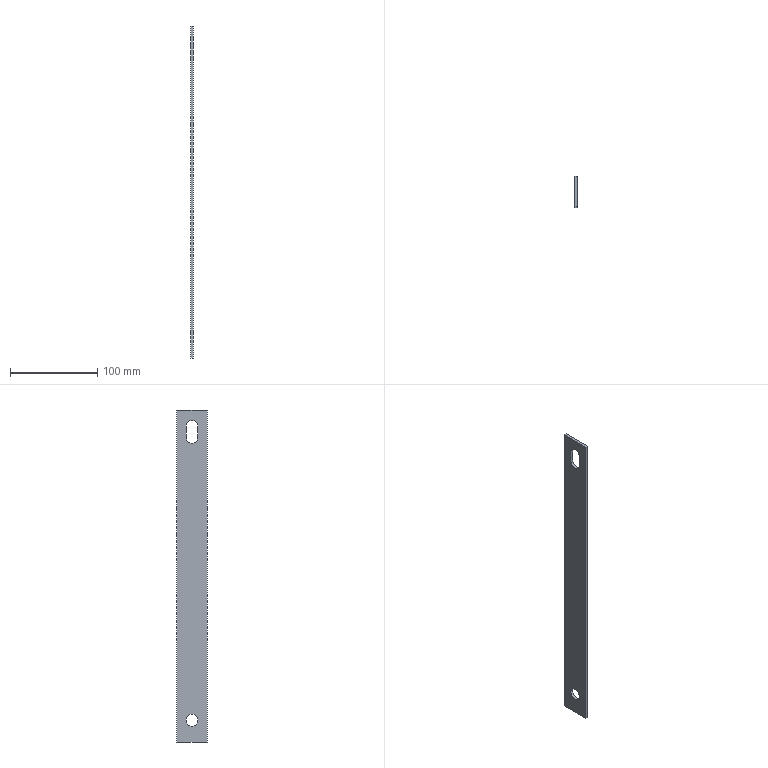Part | NX | features solid 2 | 1 solid | 11 faces | box 3 x 35 x 380 mm | volume 38535 mm3 | plane 8 | cylinder 3 | commonest cylinder face diameters 13.5 x3
STEP:
#1=CARTESIAN_POINT('',(1370.,-578.25,96.25));
#2=VERTEX_POINT('',#1);
#3=CARTESIAN_POINT('',(1370.,-591.75,96.25));
#4=VERTEX_POINT('',#3);
#5=CARTESIAN_POINT('',(1370.,-585.,96.25));
#6=DIRECTION('',(1.,0.,0.));
#7=DIRECTION('',(0.,1.,0.));
#8=AXIS2_PLACEMENT_3D('',#5,#6,#7);
#9=CIRCLE('',#8,6.75);
#10=EDGE_CURVE('',#2,#4,#9,.T.);
#11=ORIENTED_EDGE('',*,*,#10,.F.);
#12=CARTESIAN_POINT('',(1373.,-578.25,96.25));
#13=VERTEX_POINT('',#12);
#14=CARTESIAN_POINT('',(1373.,-578.25,96.25));
#15=DIRECTION('',(-1.,0.,0.));
#16=VECTOR('',#15,1000.);
#17=LINE('',#14,#16);
#18=EDGE_CURVE('',#13,#2,#17,.T.);
#19=ORIENTED_EDGE('',*,*,#18,.F.);
#20=CARTESIAN_POINT('',(1373.,-591.75,96.25));
#21=VERTEX_POINT('',#20);
#22=CARTESIAN_POINT('',(1373.,-585.,96.25));
#23=DIRECTION('',(1.,0.,0.));
#24=DIRECTION('',(0.,1.,0.));
#25=AXIS2_PLACEMENT_3D('',#22,#23,#24);
#26=CIRCLE('',#25,6.75);
#27=EDGE_CURVE('',#13,#21,#26,.T.);
#28=ORIENTED_EDGE('',*,*,#27,.T.);
#29=CARTESIAN_POINT('',(1373.,-591.75,96.25));
#30=DIRECTION('',(-1.,0.,0.));
#31=VECTOR('',#30,1000.);
#32=LINE('',#29,#31);
#33=EDGE_CURVE('',#21,#4,#32,.T.);
#34=ORIENTED_EDGE('',*,*,#33,.T.);
#35=EDGE_LOOP('',(#11,#19,#28,#34));
#36=FACE_BOUND('',#35,.T.);
#37=CARTESIAN_POINT('',(1373.,-585.,96.25));
#38=DIRECTION('',(-1.,0.,0.));
#39=DIRECTION('',(0.,1.,0.));
#40=AXIS2_PLACEMENT_3D('',#37,#38,#39);
#41=CYLINDRICAL_SURFACE('',#40,6.75);
#42=ADVANCED_FACE('',(#36),#41,.F.);
#43=CARTESIAN_POINT('',(1370.,-578.25,83.75));
#44=VERTEX_POINT('',#43);
#45=CARTESIAN_POINT('',(1370.,-578.25,96.25));
#46=DIRECTION('',(0.,0.,-1.));
#47=VECTOR('',#46,1000.);
#48=LINE('',#45,#47);
#49=EDGE_CURVE('',#2,#44,#48,.T.);
#50=ORIENTED_EDGE('',*,*,#49,.T.);
#51=CARTESIAN_POINT('',(1373.,-578.25,83.75));
#52=VERTEX_POINT('',#51);
#53=CARTESIAN_POINT('',(1373.,-578.25,83.75));
#54=DIRECTION('',(-1.,0.,0.));
#55=VECTOR('',#54,1000.);
#56=LINE('',#53,#55);
#57=EDGE_CURVE('',#52,#44,#56,.T.);
#58=ORIENTED_EDGE('',*,*,#57,.F.);
#59=CARTESIAN_POINT('',(1373.,-578.25,96.25));
#60=DIRECTION('',(0.,0.,-1.));
#61=VECTOR('',#60,1000.);
#62=LINE('',#59,#61);
#63=EDGE_CURVE('',#13,#52,#62,.T.);
#64=ORIENTED_EDGE('',*,*,#63,.F.);
#65=ORIENTED_EDGE('',*,*,#18,.T.);
#66=EDGE_LOOP('',(#50,#58,#64,#65));
#67=FACE_BOUND('',#66,.T.);
#68=CARTESIAN_POINT('',(1373.,-578.25,96.25));
#69=DIRECTION('',(0.,-1.,0.));
#70=DIRECTION('',(-1.,0.,0.));
#71=AXIS2_PLACEMENT_3D('',#68,#69,#70);
#72=PLANE('',#71);
#73=ADVANCED_FACE('',(#67),#72,.T.);
#74=CARTESIAN_POINT('',(1370.,-591.75,83.75));
#75=VERTEX_POINT('',#74);
#76=CARTESIAN_POINT('',(1370.,-585.,83.75));
#77=DIRECTION('',(1.,0.,0.));
#78=DIRECTION('',(0.,1.,0.));
#79=AXIS2_PLACEMENT_3D('',#76,#77,#78);
#80=CIRCLE('',#79,6.75);
#81=EDGE_CURVE('',#75,#44,#80,.T.);
#82=ORIENTED_EDGE('',*,*,#81,.F.);
#83=CARTESIAN_POINT('',(1373.,-591.75,83.75));
#84=VERTEX_POINT('',#83);
#85=CARTESIAN_POINT('',(1373.,-591.75,83.75));
#86=DIRECTION('',(-1.,0.,0.));
#87=VECTOR('',#86,1000.);
#88=LINE('',#85,#87);
#89=EDGE_CURVE('',#84,#75,#88,.T.);
#90=ORIENTED_EDGE('',*,*,#89,.F.);
#91=CARTESIAN_POINT('',(1373.,-585.,83.75));
#92=DIRECTION('',(1.,0.,0.));
#93=DIRECTION('',(0.,1.,0.));
#94=AXIS2_PLACEMENT_3D('',#91,#92,#93);
#95=CIRCLE('',#94,6.75);
#96=EDGE_CURVE('',#84,#52,#95,.T.);
#97=ORIENTED_EDGE('',*,*,#96,.T.);
#98=ORIENTED_EDGE('',*,*,#57,.T.);
#99=EDGE_LOOP('',(#82,#90,#97,#98));
#100=FACE_BOUND('',#99,.T.);
#101=CARTESIAN_POINT('',(1373.,-585.,83.75));
#102=DIRECTION('',(-1.,0.,0.));
#103=DIRECTION('',(0.,1.,0.));
#104=AXIS2_PLACEMENT_3D('',#101,#102,#103);
#105=CYLINDRICAL_SURFACE('',#104,6.75);
#106=ADVANCED_FACE('',(#100),#105,.F.);
#107=CARTESIAN_POINT('',(1370.,-567.5,-265.));
#108=VERTEX_POINT('',#107);
#109=CARTESIAN_POINT('',(1370.,-567.5,115.));
#110=VERTEX_POINT('',#109);
#111=CARTESIAN_POINT('',(1370.,-567.5,-130.));
#112=DIRECTION('',(0.,0.,1.));
#113=VECTOR('',#112,1000.);
#114=LINE('',#111,#113);
#115=EDGE_CURVE('',#108,#110,#114,.T.);
#116=ORIENTED_EDGE('',*,*,#115,.T.);
#117=CARTESIAN_POINT('',(1373.,-567.5,115.));
#118=VERTEX_POINT('',#117);
#119=CARTESIAN_POINT('',(1373.,-567.5,115.));
#120=DIRECTION('',(-1.,0.,0.));
#121=VECTOR('',#120,1000.);
#122=LINE('',#119,#121);
#123=EDGE_CURVE('',#118,#110,#122,.T.);
#124=ORIENTED_EDGE('',*,*,#123,.F.);
#125=CARTESIAN_POINT('',(1373.,-567.5,-265.));
#126=VERTEX_POINT('',#125);
#127=CARTESIAN_POINT('',(1373.,-567.5,-130.));
#128=DIRECTION('',(0.,0.,1.));
#129=VECTOR('',#128,1000.);
#130=LINE('',#127,#129);
#131=EDGE_CURVE('',#126,#118,#130,.T.);
#132=ORIENTED_EDGE('',*,*,#131,.F.);
#133=CARTESIAN_POINT('',(1373.,-567.5,-265.));
#134=DIRECTION('',(-1.,0.,0.));
#135=VECTOR('',#134,1000.);
#136=LINE('',#133,#135);
#137=EDGE_CURVE('',#126,#108,#136,.T.);
#138=ORIENTED_EDGE('',*,*,#137,.T.);
#139=EDGE_LOOP('',(#116,#124,#132,#138));
#140=FACE_BOUND('',#139,.T.);
#141=CARTESIAN_POINT('',(1373.,-567.5,-130.));
#142=DIRECTION('',(0.,1.,0.));
#143=DIRECTION('',(0.,0.,1.));
#144=AXIS2_PLACEMENT_3D('',#141,#142,#143);
#145=PLANE('',#144);
#146=ADVANCED_FACE('',(#140),#145,.T.);
#147=CARTESIAN_POINT('',(1370.,-602.5,115.));
#148=VERTEX_POINT('',#147);
#149=CARTESIAN_POINT('',(1370.,-567.5,115.));
#150=DIRECTION('',(0.,-1.,0.));
#151=VECTOR('',#150,1000.);
#152=LINE('',#149,#151);
#153=EDGE_CURVE('',#110,#148,#152,.T.);
#154=ORIENTED_EDGE('',*,*,#153,.T.);
#155=CARTESIAN_POINT('',(1373.,-602.5,115.));
#156=VERTEX_POINT('',#155);
#157=CARTESIAN_POINT('',(1373.,-602.5,115.));
#158=DIRECTION('',(-1.,0.,0.));
#159=VECTOR('',#158,1000.);
#160=LINE('',#157,#159);
#161=EDGE_CURVE('',#156,#148,#160,.T.);
#162=ORIENTED_EDGE('',*,*,#161,.F.);
#163=CARTESIAN_POINT('',(1373.,-567.5,115.));
#164=DIRECTION('',(0.,-1.,0.));
#165=VECTOR('',#164,1000.);
#166=LINE('',#163,#165);
#167=EDGE_CURVE('',#118,#156,#166,.T.);
#168=ORIENTED_EDGE('',*,*,#167,.F.);
#169=ORIENTED_EDGE('',*,*,#123,.T.);
#170=EDGE_LOOP('',(#154,#162,#168,#169));
#171=FACE_BOUND('',#170,.T.);
#172=CARTESIAN_POINT('',(1373.,-567.5,115.));
#173=DIRECTION('',(0.,0.,1.));
#174=DIRECTION('',(-1.,0.,0.));
#175=AXIS2_PLACEMENT_3D('',#172,#173,#174);
#176=PLANE('',#175);
#177=ADVANCED_FACE('',(#171),#176,.T.);
#178=CARTESIAN_POINT('',(1370.,-602.5,-265.));
#179=VERTEX_POINT('',#178);
#180=CARTESIAN_POINT('',(1370.,-602.5,170.));
#181=DIRECTION('',(0.,0.,-1.));
#182=VECTOR('',#181,1000.);
#183=LINE('',#180,#182);
#184=EDGE_CURVE('',#148,#179,#183,.T.);
#185=ORIENTED_EDGE('',*,*,#184,.T.);
#186=CARTESIAN_POINT('',(1373.,-602.5,-265.));
#187=VERTEX_POINT('',#186);
#188=CARTESIAN_POINT('',(1373.,-602.5,-265.));
#189=DIRECTION('',(-1.,0.,0.));
#190=VECTOR('',#189,1000.);
#191=LINE('',#188,#190);
#192=EDGE_CURVE('',#187,#179,#191,.T.);
#193=ORIENTED_EDGE('',*,*,#192,.F.);
#194=CARTESIAN_POINT('',(1373.,-602.5,170.));
#195=DIRECTION('',(0.,0.,-1.));
#196=VECTOR('',#195,1000.);
#197=LINE('',#194,#196);
#198=EDGE_CURVE('',#156,#187,#197,.T.);
#199=ORIENTED_EDGE('',*,*,#198,.F.);
#200=ORIENTED_EDGE('',*,*,#161,.T.);
#201=EDGE_LOOP('',(#185,#193,#199,#200));
#202=FACE_BOUND('',#201,.T.);
#203=CARTESIAN_POINT('',(1373.,-602.5,170.));
#204=DIRECTION('',(0.,-1.,0.));
#205=DIRECTION('',(0.,0.,-1.));
#206=AXIS2_PLACEMENT_3D('',#203,#204,#205);
#207=PLANE('',#206);
#208=ADVANCED_FACE('',(#202),#207,.T.);
#209=CARTESIAN_POINT('',(1373.,-578.25,-240.));
#210=VERTEX_POINT('',#209);
#211=CARTESIAN_POINT('',(1373.,-585.,-240.));
#212=DIRECTION('',(1.,0.,0.));
#213=DIRECTION('',(0.,1.,0.));
#214=AXIS2_PLACEMENT_3D('',#211,#212,#213);
#215=CIRCLE('',#214,6.75);
#216=EDGE_CURVE('',#210,#210,#215,.T.);
#217=ORIENTED_EDGE('',*,*,#216,.T.);
#218=EDGE_LOOP('',(#217));
#219=FACE_BOUND('',#218,.T.);
#220=CARTESIAN_POINT('',(1370.,-578.25,-240.));
#221=VERTEX_POINT('',#220);
#222=CARTESIAN_POINT('',(1370.,-585.,-240.));
#223=DIRECTION('',(1.,0.,0.));
#224=DIRECTION('',(0.,1.,0.));
#225=AXIS2_PLACEMENT_3D('',#222,#223,#224);
#226=CIRCLE('',#225,6.75);
#227=EDGE_CURVE('',#221,#221,#226,.T.);
#228=ORIENTED_EDGE('',*,*,#227,.F.);
#229=EDGE_LOOP('',(#228));
#230=FACE_BOUND('',#229,.T.);
#231=CARTESIAN_POINT('',(1373.,-585.,-240.));
#232=DIRECTION('',(-1.,0.,0.));
#233=DIRECTION('',(0.,1.,0.));
#234=AXIS2_PLACEMENT_3D('',#231,#232,#233);
#235=CYLINDRICAL_SURFACE('',#234,6.75);
#236=ADVANCED_FACE('',(#219,#230),#235,.F.);
#237=CARTESIAN_POINT('',(1370.,-602.5,-265.));
#238=DIRECTION('',(0.,1.,0.));
#239=VECTOR('',#238,1000.);
#240=LINE('',#237,#239);
#241=EDGE_CURVE('',#179,#108,#240,.T.);
#242=ORIENTED_EDGE('',*,*,#241,.T.);
#243=ORIENTED_EDGE('',*,*,#137,.F.);
#244=CARTESIAN_POINT('',(1373.,-602.5,-265.));
#245=DIRECTION('',(0.,1.,0.));
#246=VECTOR('',#245,1000.);
#247=LINE('',#244,#246);
#248=EDGE_CURVE('',#187,#126,#247,.T.);
#249=ORIENTED_EDGE('',*,*,#248,.F.);
#250=ORIENTED_EDGE('',*,*,#192,.T.);
#251=EDGE_LOOP('',(#242,#243,#249,#250));
#252=FACE_BOUND('',#251,.T.);
#253=CARTESIAN_POINT('',(1373.,-602.5,-265.));
#254=DIRECTION('',(0.,0.,-1.));
#255=DIRECTION('',(1.,0.,0.));
#256=AXIS2_PLACEMENT_3D('',#253,#254,#255);
#257=PLANE('',#256);
#258=ADVANCED_FACE('',(#252),#257,.T.);
#259=CARTESIAN_POINT('',(1370.,-591.75,83.75));
#260=DIRECTION('',(0.,0.,1.));
#261=VECTOR('',#260,1000.);
#262=LINE('',#259,#261);
#263=EDGE_CURVE('',#75,#4,#262,.T.);
#264=ORIENTED_EDGE('',*,*,#263,.T.);
#265=ORIENTED_EDGE('',*,*,#33,.F.);
#266=CARTESIAN_POINT('',(1373.,-591.75,83.75));
#267=DIRECTION('',(0.,0.,1.));
#268=VECTOR('',#267,1000.);
#269=LINE('',#266,#268);
#270=EDGE_CURVE('',#84,#21,#269,.T.);
#271=ORIENTED_EDGE('',*,*,#270,.F.);
#272=ORIENTED_EDGE('',*,*,#89,.T.);
#273=EDGE_LOOP('',(#264,#265,#271,#272));
#274=FACE_BOUND('',#273,.T.);
#275=CARTESIAN_POINT('',(1373.,-591.75,83.75));
#276=DIRECTION('',(0.,1.,0.));
#277=DIRECTION('',(1.,0.,0.));
#278=AXIS2_PLACEMENT_3D('',#275,#276,#277);
#279=PLANE('',#278);
#280=ADVANCED_FACE('',(#274),#279,.T.);
#281=ORIENTED_EDGE('',*,*,#131,.T.);
#282=ORIENTED_EDGE('',*,*,#167,.T.);
#283=ORIENTED_EDGE('',*,*,#198,.T.);
#284=ORIENTED_EDGE('',*,*,#248,.T.);
#285=EDGE_LOOP('',(#281,#282,#283,#284));
#286=FACE_BOUND('',#285,.T.);
#287=ORIENTED_EDGE('',*,*,#216,.F.);
#288=EDGE_LOOP('',(#287));
#289=FACE_BOUND('',#288,.T.);
#290=ORIENTED_EDGE('',*,*,#27,.F.);
#291=ORIENTED_EDGE('',*,*,#63,.T.);
#292=ORIENTED_EDGE('',*,*,#96,.F.);
#293=ORIENTED_EDGE('',*,*,#270,.T.);
#294=EDGE_LOOP('',(#290,#291,#292,#293));
#295=FACE_BOUND('',#294,.T.);
#296=CARTESIAN_POINT('',(1373.,-567.5,170.));
#297=DIRECTION('',(-1.,0.,0.));
#298=DIRECTION('',(0.,1.,0.));
#299=AXIS2_PLACEMENT_3D('',#296,#297,#298);
#300=PLANE('',#299);
#301=ADVANCED_FACE('',(#286,#289,#295),#300,.F.);
#302=ORIENTED_EDGE('',*,*,#115,.F.);
#303=ORIENTED_EDGE('',*,*,#241,.F.);
#304=ORIENTED_EDGE('',*,*,#184,.F.);
#305=ORIENTED_EDGE('',*,*,#153,.F.);
#306=EDGE_LOOP('',(#302,#303,#304,#305));
#307=FACE_BOUND('',#306,.T.);
#308=ORIENTED_EDGE('',*,*,#227,.T.);
#309=EDGE_LOOP('',(#308));
#310=FACE_BOUND('',#309,.T.);
#311=ORIENTED_EDGE('',*,*,#10,.T.);
#312=ORIENTED_EDGE('',*,*,#263,.F.);
#313=ORIENTED_EDGE('',*,*,#81,.T.);
#314=ORIENTED_EDGE('',*,*,#49,.F.);
#315=EDGE_LOOP('',(#311,#312,#313,#314));
#316=FACE_BOUND('',#315,.T.);
#317=CARTESIAN_POINT('',(1370.,-567.5,170.));
#318=DIRECTION('',(-1.,0.,0.));
#319=DIRECTION('',(0.,1.,0.));
#320=AXIS2_PLACEMENT_3D('',#317,#318,#319);
#321=PLANE('',#320);
#322=ADVANCED_FACE('',(#307,#310,#316),#321,.T.);
#323=CLOSED_SHELL('',(#42,#73,#106,#146,#177,#208,#236,#258,#280,#301,#322));
#324=MANIFOLD_SOLID_BREP('',#323);
#325=(LENGTH_UNIT()NAMED_UNIT(*)SI_UNIT(.MILLI.,.METRE.));
#326=UNCERTAINTY_MEASURE_WITH_UNIT(LENGTH_MEASURE(0.00001),#325,'','');
#327=(NAMED_UNIT(*)PLANE_ANGLE_UNIT()SI_UNIT($,.RADIAN.));
#328=(NAMED_UNIT(*)SI_UNIT($,.STERADIAN.)SOLID_ANGLE_UNIT());
#329=(GEOMETRIC_REPRESENTATION_CONTEXT(3)GLOBAL_UNCERTAINTY_ASSIGNED_CONTEXT((#326))GLOBAL_UNIT_ASSIGNED_CONTEXT((#325,#327,#328))REPRESENTATION_CONTEXT('',''));
#330=ADVANCED_BREP_SHAPE_REPRESENTATION('',(#324),#329);